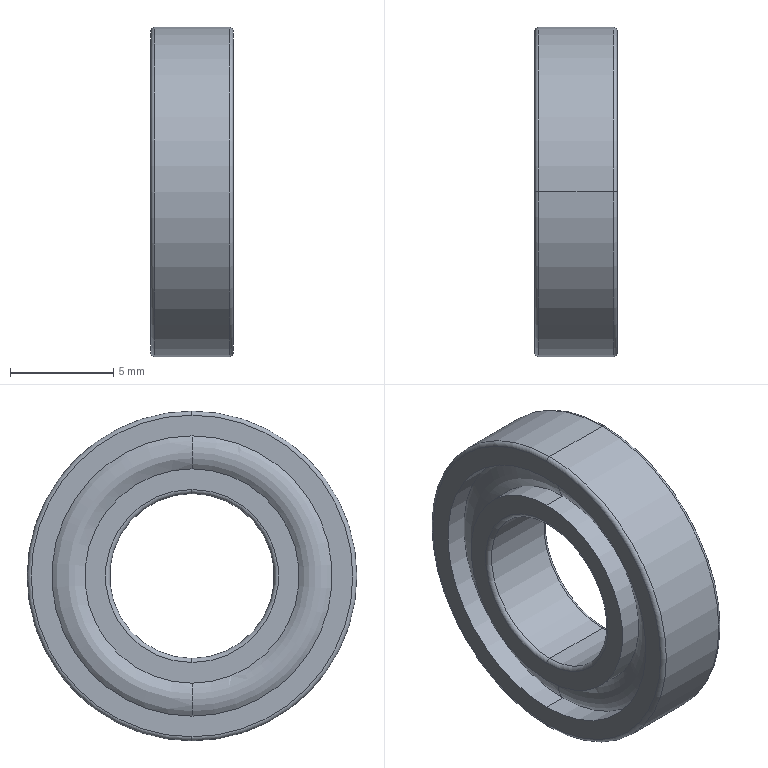Part | NX | features BREP 1 | 1 solid | 28 faces | box 4 x 16 x 16 mm | volume 493.797 mm3 | torus 12 | cylinder 12 | plane 4 | commonest cylinder face diameters 10.4 x4 13.6 x4 8 x2 16 x2
STEP:
#1=CARTESIAN_POINT('',(-2.,0.,-7.8));
#2=VERTEX_POINT('',#1);
#3=CARTESIAN_POINT('',(-2.,0.,7.8));
#4=VERTEX_POINT('',#3);
#5=CARTESIAN_POINT('',(-2.,0.,0.));
#6=DIRECTION('',(1.,0.,0.));
#7=DIRECTION('',(0.,0.,-1.));
#8=AXIS2_PLACEMENT_3D('',#5,#6,#7);
#9=CIRCLE('',#8,7.8);
#10=EDGE_CURVE('',#2,#4,#9,.T.);
#11=ORIENTED_EDGE('',*,*,#10,.T.);
#12=CARTESIAN_POINT('',(-1.8,0.,8.));
#13=VERTEX_POINT('',#12);
#14=CARTESIAN_POINT('',(-1.8,0.,7.8));
#15=DIRECTION('',(0.,1.,0.));
#16=DIRECTION('',(0.,0.,1.));
#17=AXIS2_PLACEMENT_3D('',#14,#15,#16);
#18=CIRCLE('',#17,0.2);
#19=EDGE_CURVE('',#4,#13,#18,.T.);
#20=ORIENTED_EDGE('',*,*,#19,.T.);
#21=CARTESIAN_POINT('',(-1.8,0.,-8.));
#22=VERTEX_POINT('',#21);
#23=CARTESIAN_POINT('',(-1.8,0.,0.));
#24=DIRECTION('',(1.,0.,0.));
#25=DIRECTION('',(0.,0.,-1.));
#26=AXIS2_PLACEMENT_3D('',#23,#24,#25);
#27=CIRCLE('',#26,8.);
#28=EDGE_CURVE('',#22,#13,#27,.T.);
#29=ORIENTED_EDGE('',*,*,#28,.F.);
#30=CARTESIAN_POINT('',(-1.8,0.,-7.8));
#31=DIRECTION('',(0.,-1.,0.));
#32=DIRECTION('',(0.,0.,-1.));
#33=AXIS2_PLACEMENT_3D('',#30,#31,#32);
#34=CIRCLE('',#33,0.2);
#35=EDGE_CURVE('',#2,#22,#34,.T.);
#36=ORIENTED_EDGE('',*,*,#35,.F.);
#37=EDGE_LOOP('',(#11,#20,#29,#36));
#38=FACE_BOUND('',#37,.T.);
#39=CARTESIAN_POINT('',(-1.8,0.,0.));
#40=DIRECTION('',(1.,0.,0.));
#41=DIRECTION('',(0.,0.,-1.));
#42=AXIS2_PLACEMENT_3D('',#39,#40,#41);
#43=TOROIDAL_SURFACE('',#42,7.8,0.2);
#44=ADVANCED_FACE('',(#38),#43,.T.);
#45=ORIENTED_EDGE('',*,*,#28,.T.);
#46=CARTESIAN_POINT('',(1.8,0.,8.));
#47=VERTEX_POINT('',#46);
#48=CARTESIAN_POINT('',(-20.638,0.,8.));
#49=DIRECTION('',(1.,0.,0.));
#50=VECTOR('',#49,1000.);
#51=LINE('',#48,#50);
#52=EDGE_CURVE('',#13,#47,#51,.T.);
#53=ORIENTED_EDGE('',*,*,#52,.T.);
#54=CARTESIAN_POINT('',(1.8,0.,-8.));
#55=VERTEX_POINT('',#54);
#56=CARTESIAN_POINT('',(1.8,0.,0.));
#57=DIRECTION('',(1.,0.,0.));
#58=DIRECTION('',(0.,0.,-1.));
#59=AXIS2_PLACEMENT_3D('',#56,#57,#58);
#60=CIRCLE('',#59,8.);
#61=EDGE_CURVE('',#55,#47,#60,.T.);
#62=ORIENTED_EDGE('',*,*,#61,.F.);
#63=CARTESIAN_POINT('',(-20.638,0.,-8.));
#64=DIRECTION('',(1.,0.,0.));
#65=VECTOR('',#64,1000.);
#66=LINE('',#63,#65);
#67=EDGE_CURVE('',#22,#55,#66,.T.);
#68=ORIENTED_EDGE('',*,*,#67,.F.);
#69=EDGE_LOOP('',(#45,#53,#62,#68));
#70=FACE_BOUND('',#69,.T.);
#71=CARTESIAN_POINT('',(-20.638,0.,0.));
#72=DIRECTION('',(1.,0.,0.));
#73=DIRECTION('',(0.,0.,-1.));
#74=AXIS2_PLACEMENT_3D('',#71,#72,#73);
#75=CYLINDRICAL_SURFACE('',#74,8.);
#76=ADVANCED_FACE('',(#70),#75,.T.);
#77=ORIENTED_EDGE('',*,*,#61,.T.);
#78=CARTESIAN_POINT('',(2.,0.,7.8));
#79=VERTEX_POINT('',#78);
#80=CARTESIAN_POINT('',(1.8,0.,7.8));
#81=DIRECTION('',(0.,1.,0.));
#82=DIRECTION('',(0.,0.,1.));
#83=AXIS2_PLACEMENT_3D('',#80,#81,#82);
#84=CIRCLE('',#83,0.2);
#85=EDGE_CURVE('',#47,#79,#84,.T.);
#86=ORIENTED_EDGE('',*,*,#85,.T.);
#87=CARTESIAN_POINT('',(2.,0.,-7.8));
#88=VERTEX_POINT('',#87);
#89=CARTESIAN_POINT('',(2.,0.,0.));
#90=DIRECTION('',(1.,0.,0.));
#91=DIRECTION('',(0.,0.,-1.));
#92=AXIS2_PLACEMENT_3D('',#89,#90,#91);
#93=CIRCLE('',#92,7.8);
#94=EDGE_CURVE('',#88,#79,#93,.T.);
#95=ORIENTED_EDGE('',*,*,#94,.F.);
#96=CARTESIAN_POINT('',(1.8,0.,-7.8));
#97=DIRECTION('',(0.,-1.,0.));
#98=DIRECTION('',(0.,0.,-1.));
#99=AXIS2_PLACEMENT_3D('',#96,#97,#98);
#100=CIRCLE('',#99,0.2);
#101=EDGE_CURVE('',#55,#88,#100,.T.);
#102=ORIENTED_EDGE('',*,*,#101,.F.);
#103=EDGE_LOOP('',(#77,#86,#95,#102));
#104=FACE_BOUND('',#103,.T.);
#105=CARTESIAN_POINT('',(1.8,0.,0.));
#106=DIRECTION('',(1.,0.,0.));
#107=DIRECTION('',(0.,0.,-1.));
#108=AXIS2_PLACEMENT_3D('',#105,#106,#107);
#109=TOROIDAL_SURFACE('',#108,7.8,0.2);
#110=ADVANCED_FACE('',(#104),#109,.T.);
#111=CARTESIAN_POINT('',(-2.,0.,6.8));
#112=VERTEX_POINT('',#111);
#113=CARTESIAN_POINT('',(-2.,0.,-6.8));
#114=VERTEX_POINT('',#113);
#115=CARTESIAN_POINT('',(-2.,0.,0.));
#116=DIRECTION('',(1.,0.,0.));
#117=DIRECTION('',(0.,0.,-1.));
#118=AXIS2_PLACEMENT_3D('',#115,#116,#117);
#119=CIRCLE('',#118,6.8);
#120=EDGE_CURVE('',#112,#114,#119,.T.);
#121=ORIENTED_EDGE('',*,*,#120,.F.);
#122=CARTESIAN_POINT('',(-0.8944,0.,6.8));
#123=VERTEX_POINT('',#122);
#124=CARTESIAN_POINT('',(-20.638,0.,6.8));
#125=DIRECTION('',(1.,0.,0.));
#126=VECTOR('',#125,1000.);
#127=LINE('',#124,#126);
#128=EDGE_CURVE('',#112,#123,#127,.T.);
#129=ORIENTED_EDGE('',*,*,#128,.T.);
#130=CARTESIAN_POINT('',(-0.8944,0.,-6.8));
#131=VERTEX_POINT('',#130);
#132=CARTESIAN_POINT('',(-0.8944,0.,0.));
#133=DIRECTION('',(-1.,0.,0.));
#134=DIRECTION('',(0.,0.,-1.));
#135=AXIS2_PLACEMENT_3D('',#132,#133,#134);
#136=CIRCLE('',#135,6.8);
#137=EDGE_CURVE('',#131,#123,#136,.T.);
#138=ORIENTED_EDGE('',*,*,#137,.F.);
#139=CARTESIAN_POINT('',(-20.638,0.,-6.8));
#140=DIRECTION('',(1.,0.,0.));
#141=VECTOR('',#140,1000.);
#142=LINE('',#139,#141);
#143=EDGE_CURVE('',#114,#131,#142,.T.);
#144=ORIENTED_EDGE('',*,*,#143,.F.);
#145=EDGE_LOOP('',(#121,#129,#138,#144));
#146=FACE_BOUND('',#145,.T.);
#147=CARTESIAN_POINT('',(-20.638,0.,0.));
#148=DIRECTION('',(1.,0.,0.));
#149=DIRECTION('',(0.,0.,-1.));
#150=AXIS2_PLACEMENT_3D('',#147,#148,#149);
#151=CYLINDRICAL_SURFACE('',#150,6.8);
#152=ADVANCED_FACE('',(#146),#151,.F.);
#153=CARTESIAN_POINT('',(0.8944,0.,6.8));
#154=VERTEX_POINT('',#153);
#155=CARTESIAN_POINT('',(0.8944,0.,-6.8));
#156=VERTEX_POINT('',#155);
#157=CARTESIAN_POINT('',(0.8944,0.,0.));
#158=DIRECTION('',(1.,0.,0.));
#159=DIRECTION('',(0.,0.,1.));
#160=AXIS2_PLACEMENT_3D('',#157,#158,#159);
#161=CIRCLE('',#160,6.8);
#162=EDGE_CURVE('',#154,#156,#161,.T.);
#163=ORIENTED_EDGE('',*,*,#162,.F.);
#164=CARTESIAN_POINT('',(2.,0.,6.8));
#165=VERTEX_POINT('',#164);
#166=CARTESIAN_POINT('',(-20.638,0.,6.8));
#167=DIRECTION('',(1.,0.,0.));
#168=VECTOR('',#167,1000.);
#169=LINE('',#166,#168);
#170=EDGE_CURVE('',#154,#165,#169,.T.);
#171=ORIENTED_EDGE('',*,*,#170,.T.);
#172=CARTESIAN_POINT('',(2.,0.,-6.8));
#173=VERTEX_POINT('',#172);
#174=CARTESIAN_POINT('',(2.,0.,0.));
#175=DIRECTION('',(1.,0.,0.));
#176=DIRECTION('',(0.,0.,-1.));
#177=AXIS2_PLACEMENT_3D('',#174,#175,#176);
#178=CIRCLE('',#177,6.8);
#179=EDGE_CURVE('',#165,#173,#178,.T.);
#180=ORIENTED_EDGE('',*,*,#179,.T.);
#181=CARTESIAN_POINT('',(-20.638,0.,-6.8));
#182=DIRECTION('',(1.,0.,0.));
#183=VECTOR('',#182,1000.);
#184=LINE('',#181,#183);
#185=EDGE_CURVE('',#156,#173,#184,.T.);
#186=ORIENTED_EDGE('',*,*,#185,.F.);
#187=EDGE_LOOP('',(#163,#171,#180,#186));
#188=FACE_BOUND('',#187,.T.);
#189=CARTESIAN_POINT('',(-20.638,0.,0.));
#190=DIRECTION('',(1.,0.,0.));
#191=DIRECTION('',(0.,0.,-1.));
#192=AXIS2_PLACEMENT_3D('',#189,#190,#191);
#193=CYLINDRICAL_SURFACE('',#192,6.8);
#194=ADVANCED_FACE('',(#188),#193,.F.);
#195=CARTESIAN_POINT('',(-0.8944,0.,0.));
#196=DIRECTION('',(-1.,0.,0.));
#197=DIRECTION('',(0.,0.,-1.));
#198=AXIS2_PLACEMENT_3D('',#195,#196,#197);
#199=CIRCLE('',#198,6.8);
#200=EDGE_CURVE('',#123,#131,#199,.T.);
#201=ORIENTED_EDGE('',*,*,#200,.T.);
#202=CARTESIAN_POINT('',(-0.8944,0.,-5.2));
#203=VERTEX_POINT('',#202);
#204=CARTESIAN_POINT('',(0.,0.,-6.));
#205=DIRECTION('',(0.,1.,0.));
#206=DIRECTION('',(0.,0.,1.));
#207=AXIS2_PLACEMENT_3D('',#204,#205,#206);
#208=CIRCLE('',#207,1.2);
#209=EDGE_CURVE('',#203,#131,#208,.F.);
#210=ORIENTED_EDGE('',*,*,#209,.F.);
#211=CARTESIAN_POINT('',(-0.8944,0.,5.2));
#212=VERTEX_POINT('',#211);
#213=CARTESIAN_POINT('',(-0.8944,0.,0.));
#214=DIRECTION('',(1.,0.,0.));
#215=DIRECTION('',(0.,0.,-1.));
#216=AXIS2_PLACEMENT_3D('',#213,#214,#215);
#217=CIRCLE('',#216,5.2);
#218=EDGE_CURVE('',#203,#212,#217,.T.);
#219=ORIENTED_EDGE('',*,*,#218,.T.);
#220=CARTESIAN_POINT('',(0.,0.,6.));
#221=DIRECTION('',(0.,-1.,0.));
#222=DIRECTION('',(0.,0.,-1.));
#223=AXIS2_PLACEMENT_3D('',#220,#221,#222);
#224=CIRCLE('',#223,1.2);
#225=EDGE_CURVE('',#212,#123,#224,.F.);
#226=ORIENTED_EDGE('',*,*,#225,.T.);
#227=EDGE_LOOP('',(#201,#210,#219,#226));
#228=FACE_BOUND('',#227,.T.);
#229=CARTESIAN_POINT('',(0.,0.,0.));
#230=DIRECTION('',(-1.,0.,0.));
#231=DIRECTION('',(0.,0.,1.));
#232=AXIS2_PLACEMENT_3D('',#229,#230,#231);
#233=TOROIDAL_SURFACE('',#232,6.,1.2);
#234=ADVANCED_FACE('',(#228),#233,.T.);
#235=CARTESIAN_POINT('',(-1.8,0.,-4.));
#236=VERTEX_POINT('',#235);
#237=CARTESIAN_POINT('',(-1.8,0.,4.));
#238=VERTEX_POINT('',#237);
#239=CARTESIAN_POINT('',(-1.8,0.,0.));
#240=DIRECTION('',(1.,0.,0.));
#241=DIRECTION('',(0.,0.,-1.));
#242=AXIS2_PLACEMENT_3D('',#239,#240,#241);
#243=CIRCLE('',#242,4.);
#244=EDGE_CURVE('',#236,#238,#243,.T.);
#245=ORIENTED_EDGE('',*,*,#244,.T.);
#246=CARTESIAN_POINT('',(-2.,0.,4.2));
#247=VERTEX_POINT('',#246);
#248=CARTESIAN_POINT('',(-1.8,0.,4.2));
#249=DIRECTION('',(0.,1.,0.));
#250=DIRECTION('',(0.,0.,1.));
#251=AXIS2_PLACEMENT_3D('',#248,#249,#250);
#252=CIRCLE('',#251,0.2);
#253=EDGE_CURVE('',#238,#247,#252,.T.);
#254=ORIENTED_EDGE('',*,*,#253,.T.);
#255=CARTESIAN_POINT('',(-2.,0.,-4.2));
#256=VERTEX_POINT('',#255);
#257=CARTESIAN_POINT('',(-2.,0.,0.));
#258=DIRECTION('',(1.,0.,0.));
#259=DIRECTION('',(0.,0.,-1.));
#260=AXIS2_PLACEMENT_3D('',#257,#258,#259);
#261=CIRCLE('',#260,4.2);
#262=EDGE_CURVE('',#256,#247,#261,.T.);
#263=ORIENTED_EDGE('',*,*,#262,.F.);
#264=CARTESIAN_POINT('',(-1.8,0.,-4.2));
#265=DIRECTION('',(0.,-1.,0.));
#266=DIRECTION('',(0.,0.,-1.));
#267=AXIS2_PLACEMENT_3D('',#264,#265,#266);
#268=CIRCLE('',#267,0.2);
#269=EDGE_CURVE('',#236,#256,#268,.T.);
#270=ORIENTED_EDGE('',*,*,#269,.F.);
#271=EDGE_LOOP('',(#245,#254,#263,#270));
#272=FACE_BOUND('',#271,.T.);
#273=CARTESIAN_POINT('',(-1.8,0.,0.));
#274=DIRECTION('',(1.,0.,0.));
#275=DIRECTION('',(0.,0.,-1.));
#276=AXIS2_PLACEMENT_3D('',#273,#274,#275);
#277=TOROIDAL_SURFACE('',#276,4.2,0.2);
#278=ADVANCED_FACE('',(#272),#277,.T.);
#279=CARTESIAN_POINT('',(-1.8,0.,0.));
#280=DIRECTION('',(1.,0.,0.));
#281=DIRECTION('',(0.,0.,-1.));
#282=AXIS2_PLACEMENT_3D('',#279,#280,#281);
#283=CIRCLE('',#282,4.);
#284=EDGE_CURVE('',#238,#236,#283,.T.);
#285=ORIENTED_EDGE('',*,*,#284,.F.);
#286=CARTESIAN_POINT('',(1.8,0.,4.));
#287=VERTEX_POINT('',#286);
#288=CARTESIAN_POINT('',(-20.638,0.,4.));
#289=DIRECTION('',(1.,0.,0.));
#290=VECTOR('',#289,1000.);
#291=LINE('',#288,#290);
#292=EDGE_CURVE('',#238,#287,#291,.T.);
#293=ORIENTED_EDGE('',*,*,#292,.T.);
#294=CARTESIAN_POINT('',(1.8,0.,-4.));
#295=VERTEX_POINT('',#294);
#296=CARTESIAN_POINT('',(1.8,0.,0.));
#297=DIRECTION('',(1.,0.,0.));
#298=DIRECTION('',(0.,0.,-1.));
#299=AXIS2_PLACEMENT_3D('',#296,#297,#298);
#300=CIRCLE('',#299,4.);
#301=EDGE_CURVE('',#287,#295,#300,.T.);
#302=ORIENTED_EDGE('',*,*,#301,.T.);
#303=CARTESIAN_POINT('',(-20.638,0.,-4.));
#304=DIRECTION('',(1.,0.,0.));
#305=VECTOR('',#304,1000.);
#306=LINE('',#303,#305);
#307=EDGE_CURVE('',#236,#295,#306,.T.);
#308=ORIENTED_EDGE('',*,*,#307,.F.);
#309=EDGE_LOOP('',(#285,#293,#302,#308));
#310=FACE_BOUND('',#309,.T.);
#311=CARTESIAN_POINT('',(-20.638,0.,0.));
#312=DIRECTION('',(1.,0.,0.));
#313=DIRECTION('',(0.,0.,-1.));
#314=AXIS2_PLACEMENT_3D('',#311,#312,#313);
#315=CYLINDRICAL_SURFACE('',#314,4.);
#316=ADVANCED_FACE('',(#310),#315,.F.);
#317=CARTESIAN_POINT('',(2.,0.,-4.2));
#318=VERTEX_POINT('',#317);
#319=CARTESIAN_POINT('',(2.,0.,4.2));
#320=VERTEX_POINT('',#319);
#321=CARTESIAN_POINT('',(2.,0.,0.));
#322=DIRECTION('',(1.,0.,0.));
#323=DIRECTION('',(0.,0.,-1.));
#324=AXIS2_PLACEMENT_3D('',#321,#322,#323);
#325=CIRCLE('',#324,4.2);
#326=EDGE_CURVE('',#318,#320,#325,.T.);
#327=ORIENTED_EDGE('',*,*,#326,.T.);
#328=CARTESIAN_POINT('',(1.8,0.,4.2));
#329=DIRECTION('',(0.,1.,0.));
#330=DIRECTION('',(0.,0.,1.));
#331=AXIS2_PLACEMENT_3D('',#328,#329,#330);
#332=CIRCLE('',#331,0.2);
#333=EDGE_CURVE('',#320,#287,#332,.T.);
#334=ORIENTED_EDGE('',*,*,#333,.T.);
#335=CARTESIAN_POINT('',(1.8,0.,0.));
#336=DIRECTION('',(1.,0.,0.));
#337=DIRECTION('',(0.,0.,-1.));
#338=AXIS2_PLACEMENT_3D('',#335,#336,#337);
#339=CIRCLE('',#338,4.);
#340=EDGE_CURVE('',#295,#287,#339,.T.);
#341=ORIENTED_EDGE('',*,*,#340,.F.);
#342=CARTESIAN_POINT('',(1.8,0.,-4.2));
#343=DIRECTION('',(0.,-1.,0.));
#344=DIRECTION('',(0.,0.,-1.));
#345=AXIS2_PLACEMENT_3D('',#342,#343,#344);
#346=CIRCLE('',#345,0.2);
#347=EDGE_CURVE('',#318,#295,#346,.T.);
#348=ORIENTED_EDGE('',*,*,#347,.F.);
#349=EDGE_LOOP('',(#327,#334,#341,#348));
#350=FACE_BOUND('',#349,.T.);
#351=CARTESIAN_POINT('',(1.8,0.,0.));
#352=DIRECTION('',(1.,0.,0.));
#353=DIRECTION('',(0.,0.,-1.));
#354=AXIS2_PLACEMENT_3D('',#351,#352,#353);
#355=TOROIDAL_SURFACE('',#354,4.2,0.2);
#356=ADVANCED_FACE('',(#350),#355,.T.);
#357=CARTESIAN_POINT('',(-2.,0.,-5.2));
#358=VERTEX_POINT('',#357);
#359=CARTESIAN_POINT('',(-2.,0.,5.2));
#360=VERTEX_POINT('',#359);
#361=CARTESIAN_POINT('',(-2.,0.,0.));
#362=DIRECTION('',(1.,0.,0.));
#363=DIRECTION('',(0.,0.,-1.));
#364=AXIS2_PLACEMENT_3D('',#361,#362,#363);
#365=CIRCLE('',#364,5.2);
#366=EDGE_CURVE('',#358,#360,#365,.T.);
#367=ORIENTED_EDGE('',*,*,#366,.T.);
#368=CARTESIAN_POINT('',(-20.638,0.,5.2));
#369=DIRECTION('',(1.,0.,0.));
#370=VECTOR('',#369,1000.);
#371=LINE('',#368,#370);
#372=EDGE_CURVE('',#360,#212,#371,.T.);
#373=ORIENTED_EDGE('',*,*,#372,.T.);
#374=ORIENTED_EDGE('',*,*,#218,.F.);
#375=CARTESIAN_POINT('',(-20.638,0.,-5.2));
#376=DIRECTION('',(1.,0.,0.));
#377=VECTOR('',#376,1000.);
#378=LINE('',#375,#377);
#379=EDGE_CURVE('',#358,#203,#378,.T.);
#380=ORIENTED_EDGE('',*,*,#379,.F.);
#381=EDGE_LOOP('',(#367,#373,#374,#380));
#382=FACE_BOUND('',#381,.T.);
#383=CARTESIAN_POINT('',(-20.638,0.,0.));
#384=DIRECTION('',(1.,0.,0.));
#385=DIRECTION('',(0.,0.,-1.));
#386=AXIS2_PLACEMENT_3D('',#383,#384,#385);
#387=CYLINDRICAL_SURFACE('',#386,5.2);
#388=ADVANCED_FACE('',(#382),#387,.T.);
#389=CARTESIAN_POINT('',(0.8944,0.,5.2));
#390=VERTEX_POINT('',#389);
#391=CARTESIAN_POINT('',(0.8944,0.,-5.2));
#392=VERTEX_POINT('',#391);
#393=CARTESIAN_POINT('',(0.8944,0.,0.));
#394=DIRECTION('',(-1.,0.,0.));
#395=DIRECTION('',(0.,0.,1.));
#396=AXIS2_PLACEMENT_3D('',#393,#394,#395);
#397=CIRCLE('',#396,5.2);
#398=EDGE_CURVE('',#390,#392,#397,.T.);
#399=ORIENTED_EDGE('',*,*,#398,.F.);
#400=CARTESIAN_POINT('',(2.,0.,5.2));
#401=VERTEX_POINT('',#400);
#402=CARTESIAN_POINT('',(-20.638,0.,5.2));
#403=DIRECTION('',(1.,0.,0.));
#404=VECTOR('',#403,1000.);
#405=LINE('',#402,#404);
#406=EDGE_CURVE('',#390,#401,#405,.T.);
#407=ORIENTED_EDGE('',*,*,#406,.T.);
#408=CARTESIAN_POINT('',(2.,0.,-5.2));
#409=VERTEX_POINT('',#408);
#410=CARTESIAN_POINT('',(2.,0.,0.));
#411=DIRECTION('',(1.,0.,0.));
#412=DIRECTION('',(0.,0.,-1.));
#413=AXIS2_PLACEMENT_3D('',#410,#411,#412);
#414=CIRCLE('',#413,5.2);
#415=EDGE_CURVE('',#409,#401,#414,.T.);
#416=ORIENTED_EDGE('',*,*,#415,.F.);
#417=CARTESIAN_POINT('',(-20.638,0.,-5.2));
#418=DIRECTION('',(1.,0.,0.));
#419=VECTOR('',#418,1000.);
#420=LINE('',#417,#419);
#421=EDGE_CURVE('',#392,#409,#420,.T.);
#422=ORIENTED_EDGE('',*,*,#421,.F.);
#423=EDGE_LOOP('',(#399,#407,#416,#422));
#424=FACE_BOUND('',#423,.T.);
#425=CARTESIAN_POINT('',(-20.638,0.,0.));
#426=DIRECTION('',(1.,0.,0.));
#427=DIRECTION('',(0.,0.,-1.));
#428=AXIS2_PLACEMENT_3D('',#425,#426,#427);
#429=CYLINDRICAL_SURFACE('',#428,5.2);
#430=ADVANCED_FACE('',(#424),#429,.T.);
#431=ORIENTED_EDGE('',*,*,#398,.T.);
#432=CARTESIAN_POINT('',(0.,0.,-6.));
#433=DIRECTION('',(0.,1.,0.));
#434=DIRECTION('',(0.,0.,1.));
#435=AXIS2_PLACEMENT_3D('',#432,#433,#434);
#436=CIRCLE('',#435,1.2);
#437=EDGE_CURVE('',#156,#392,#436,.F.);
#438=ORIENTED_EDGE('',*,*,#437,.F.);
#439=CARTESIAN_POINT('',(0.8944,0.,0.));
#440=DIRECTION('',(1.,0.,0.));
#441=DIRECTION('',(0.,0.,1.));
#442=AXIS2_PLACEMENT_3D('',#439,#440,#441);
#443=CIRCLE('',#442,6.8);
#444=EDGE_CURVE('',#156,#154,#443,.T.);
#445=ORIENTED_EDGE('',*,*,#444,.T.);
#446=CARTESIAN_POINT('',(0.,0.,6.));
#447=DIRECTION('',(0.,-1.,0.));
#448=DIRECTION('',(0.,0.,-1.));
#449=AXIS2_PLACEMENT_3D('',#446,#447,#448);
#450=CIRCLE('',#449,1.2);
#451=EDGE_CURVE('',#154,#390,#450,.F.);
#452=ORIENTED_EDGE('',*,*,#451,.T.);
#453=EDGE_LOOP('',(#431,#438,#445,#452));
#454=FACE_BOUND('',#453,.T.);
#455=CARTESIAN_POINT('',(0.,0.,0.));
#456=DIRECTION('',(-1.,0.,0.));
#457=DIRECTION('',(0.,0.,1.));
#458=AXIS2_PLACEMENT_3D('',#455,#456,#457);
#459=TOROIDAL_SURFACE('',#458,6.,1.2);
#460=ADVANCED_FACE('',(#454),#459,.T.);
#461=ORIENTED_EDGE('',*,*,#437,.T.);
#462=CARTESIAN_POINT('',(0.8944,0.,0.));
#463=DIRECTION('',(-1.,0.,0.));
#464=DIRECTION('',(0.,0.,1.));
#465=AXIS2_PLACEMENT_3D('',#462,#463,#464);
#466=CIRCLE('',#465,5.2);
#467=EDGE_CURVE('',#392,#390,#466,.T.);
#468=ORIENTED_EDGE('',*,*,#467,.T.);
#469=ORIENTED_EDGE('',*,*,#451,.F.);
#470=ORIENTED_EDGE('',*,*,#162,.T.);
#471=EDGE_LOOP('',(#461,#468,#469,#470));
#472=FACE_BOUND('',#471,.T.);
#473=CARTESIAN_POINT('',(0.,0.,0.));
#474=DIRECTION('',(-1.,0.,0.));
#475=DIRECTION('',(0.,0.,1.));
#476=AXIS2_PLACEMENT_3D('',#473,#474,#475);
#477=TOROIDAL_SURFACE('',#476,6.,1.2);
#478=ADVANCED_FACE('',(#472),#477,.T.);
#479=ORIENTED_EDGE('',*,*,#406,.F.);
#480=ORIENTED_EDGE('',*,*,#467,.F.);
#481=ORIENTED_EDGE('',*,*,#421,.T.);
#482=CARTESIAN_POINT('',(2.,0.,0.));
#483=DIRECTION('',(1.,0.,0.));
#484=DIRECTION('',(0.,0.,-1.));
#485=AXIS2_PLACEMENT_3D('',#482,#483,#484);
#486=CIRCLE('',#485,5.2);
#487=EDGE_CURVE('',#401,#409,#486,.T.);
#488=ORIENTED_EDGE('',*,*,#487,.F.);
#489=EDGE_LOOP('',(#479,#480,#481,#488));
#490=FACE_BOUND('',#489,.T.);
#491=CARTESIAN_POINT('',(-20.638,0.,0.));
#492=DIRECTION('',(1.,0.,0.));
#493=DIRECTION('',(0.,0.,-1.));
#494=AXIS2_PLACEMENT_3D('',#491,#492,#493);
#495=CYLINDRICAL_SURFACE('',#494,5.2);
#496=ADVANCED_FACE('',(#490),#495,.T.);
#497=ORIENTED_EDGE('',*,*,#372,.F.);
#498=CARTESIAN_POINT('',(-2.,0.,0.));
#499=DIRECTION('',(1.,0.,0.));
#500=DIRECTION('',(0.,0.,-1.));
#501=AXIS2_PLACEMENT_3D('',#498,#499,#500);
#502=CIRCLE('',#501,5.2);
#503=EDGE_CURVE('',#360,#358,#502,.T.);
#504=ORIENTED_EDGE('',*,*,#503,.T.);
#505=ORIENTED_EDGE('',*,*,#379,.T.);
#506=CARTESIAN_POINT('',(-0.8944,0.,0.));
#507=DIRECTION('',(1.,0.,0.));
#508=DIRECTION('',(0.,0.,-1.));
#509=AXIS2_PLACEMENT_3D('',#506,#507,#508);
#510=CIRCLE('',#509,5.2);
#511=EDGE_CURVE('',#212,#203,#510,.T.);
#512=ORIENTED_EDGE('',*,*,#511,.F.);
#513=EDGE_LOOP('',(#497,#504,#505,#512));
#514=FACE_BOUND('',#513,.T.);
#515=CARTESIAN_POINT('',(-20.638,0.,0.));
#516=DIRECTION('',(1.,0.,0.));
#517=DIRECTION('',(0.,0.,-1.));
#518=AXIS2_PLACEMENT_3D('',#515,#516,#517);
#519=CYLINDRICAL_SURFACE('',#518,5.2);
#520=ADVANCED_FACE('',(#514),#519,.T.);
#521=ORIENTED_EDGE('',*,*,#415,.T.);
#522=ORIENTED_EDGE('',*,*,#487,.T.);
#523=EDGE_LOOP('',(#521,#522));
#524=FACE_BOUND('',#523,.T.);
#525=ORIENTED_EDGE('',*,*,#326,.F.);
#526=CARTESIAN_POINT('',(2.,0.,0.));
#527=DIRECTION('',(1.,0.,0.));
#528=DIRECTION('',(0.,0.,-1.));
#529=AXIS2_PLACEMENT_3D('',#526,#527,#528);
#530=CIRCLE('',#529,4.2);
#531=EDGE_CURVE('',#320,#318,#530,.T.);
#532=ORIENTED_EDGE('',*,*,#531,.F.);
#533=EDGE_LOOP('',(#525,#532));
#534=FACE_BOUND('',#533,.T.);
#535=CARTESIAN_POINT('',(2.,4.2,0.));
#536=DIRECTION('',(1.,0.,0.));
#537=DIRECTION('',(0.,1.,0.));
#538=AXIS2_PLACEMENT_3D('',#535,#536,#537);
#539=PLANE('',#538);
#540=ADVANCED_FACE('',(#524,#534),#539,.T.);
#541=ORIENTED_EDGE('',*,*,#333,.F.);
#542=ORIENTED_EDGE('',*,*,#531,.T.);
#543=ORIENTED_EDGE('',*,*,#347,.T.);
#544=ORIENTED_EDGE('',*,*,#301,.F.);
#545=EDGE_LOOP('',(#541,#542,#543,#544));
#546=FACE_BOUND('',#545,.T.);
#547=CARTESIAN_POINT('',(1.8,0.,0.));
#548=DIRECTION('',(1.,0.,0.));
#549=DIRECTION('',(0.,0.,-1.));
#550=AXIS2_PLACEMENT_3D('',#547,#548,#549);
#551=TOROIDAL_SURFACE('',#550,4.2,0.2);
#552=ADVANCED_FACE('',(#546),#551,.T.);
#553=ORIENTED_EDGE('',*,*,#292,.F.);
#554=ORIENTED_EDGE('',*,*,#244,.F.);
#555=ORIENTED_EDGE('',*,*,#307,.T.);
#556=ORIENTED_EDGE('',*,*,#340,.T.);
#557=EDGE_LOOP('',(#553,#554,#555,#556));
#558=FACE_BOUND('',#557,.T.);
#559=CARTESIAN_POINT('',(-20.638,0.,0.));
#560=DIRECTION('',(1.,0.,0.));
#561=DIRECTION('',(0.,0.,-1.));
#562=AXIS2_PLACEMENT_3D('',#559,#560,#561);
#563=CYLINDRICAL_SURFACE('',#562,4.);
#564=ADVANCED_FACE('',(#558),#563,.F.);
#565=ORIENTED_EDGE('',*,*,#253,.F.);
#566=ORIENTED_EDGE('',*,*,#284,.T.);
#567=ORIENTED_EDGE('',*,*,#269,.T.);
#568=CARTESIAN_POINT('',(-2.,0.,0.));
#569=DIRECTION('',(1.,0.,0.));
#570=DIRECTION('',(0.,0.,-1.));
#571=AXIS2_PLACEMENT_3D('',#568,#569,#570);
#572=CIRCLE('',#571,4.2);
#573=EDGE_CURVE('',#247,#256,#572,.T.);
#574=ORIENTED_EDGE('',*,*,#573,.F.);
#575=EDGE_LOOP('',(#565,#566,#567,#574));
#576=FACE_BOUND('',#575,.T.);
#577=CARTESIAN_POINT('',(-1.8,0.,0.));
#578=DIRECTION('',(1.,0.,0.));
#579=DIRECTION('',(0.,0.,-1.));
#580=AXIS2_PLACEMENT_3D('',#577,#578,#579);
#581=TOROIDAL_SURFACE('',#580,4.2,0.2);
#582=ADVANCED_FACE('',(#576),#581,.T.);
#583=ORIENTED_EDGE('',*,*,#366,.F.);
#584=ORIENTED_EDGE('',*,*,#503,.F.);
#585=EDGE_LOOP('',(#583,#584));
#586=FACE_BOUND('',#585,.T.);
#587=ORIENTED_EDGE('',*,*,#262,.T.);
#588=ORIENTED_EDGE('',*,*,#573,.T.);
#589=EDGE_LOOP('',(#587,#588));
#590=FACE_BOUND('',#589,.T.);
#591=CARTESIAN_POINT('',(-2.,5.2,0.));
#592=DIRECTION('',(-1.,0.,0.));
#593=DIRECTION('',(0.,1.,0.));
#594=AXIS2_PLACEMENT_3D('',#591,#592,#593);
#595=PLANE('',#594);
#596=ADVANCED_FACE('',(#586,#590),#595,.T.);
#597=ORIENTED_EDGE('',*,*,#209,.T.);
#598=ORIENTED_EDGE('',*,*,#137,.T.);
#599=ORIENTED_EDGE('',*,*,#225,.F.);
#600=ORIENTED_EDGE('',*,*,#511,.T.);
#601=EDGE_LOOP('',(#597,#598,#599,#600));
#602=FACE_BOUND('',#601,.T.);
#603=CARTESIAN_POINT('',(0.,0.,0.));
#604=DIRECTION('',(-1.,0.,0.));
#605=DIRECTION('',(0.,0.,1.));
#606=AXIS2_PLACEMENT_3D('',#603,#604,#605);
#607=TOROIDAL_SURFACE('',#606,6.,1.2);
#608=ADVANCED_FACE('',(#602),#607,.T.);
#609=ORIENTED_EDGE('',*,*,#170,.F.);
#610=ORIENTED_EDGE('',*,*,#444,.F.);
#611=ORIENTED_EDGE('',*,*,#185,.T.);
#612=CARTESIAN_POINT('',(2.,0.,0.));
#613=DIRECTION('',(1.,0.,0.));
#614=DIRECTION('',(0.,0.,-1.));
#615=AXIS2_PLACEMENT_3D('',#612,#613,#614);
#616=CIRCLE('',#615,6.8);
#617=EDGE_CURVE('',#173,#165,#616,.T.);
#618=ORIENTED_EDGE('',*,*,#617,.T.);
#619=EDGE_LOOP('',(#609,#610,#611,#618));
#620=FACE_BOUND('',#619,.T.);
#621=CARTESIAN_POINT('',(-20.638,0.,0.));
#622=DIRECTION('',(1.,0.,0.));
#623=DIRECTION('',(0.,0.,-1.));
#624=AXIS2_PLACEMENT_3D('',#621,#622,#623);
#625=CYLINDRICAL_SURFACE('',#624,6.8);
#626=ADVANCED_FACE('',(#620),#625,.F.);
#627=ORIENTED_EDGE('',*,*,#128,.F.);
#628=CARTESIAN_POINT('',(-2.,0.,0.));
#629=DIRECTION('',(1.,0.,0.));
#630=DIRECTION('',(0.,0.,-1.));
#631=AXIS2_PLACEMENT_3D('',#628,#629,#630);
#632=CIRCLE('',#631,6.8);
#633=EDGE_CURVE('',#114,#112,#632,.T.);
#634=ORIENTED_EDGE('',*,*,#633,.F.);
#635=ORIENTED_EDGE('',*,*,#143,.T.);
#636=ORIENTED_EDGE('',*,*,#200,.F.);
#637=EDGE_LOOP('',(#627,#634,#635,#636));
#638=FACE_BOUND('',#637,.T.);
#639=CARTESIAN_POINT('',(-20.638,0.,0.));
#640=DIRECTION('',(1.,0.,0.));
#641=DIRECTION('',(0.,0.,-1.));
#642=AXIS2_PLACEMENT_3D('',#639,#640,#641);
#643=CYLINDRICAL_SURFACE('',#642,6.8);
#644=ADVANCED_FACE('',(#638),#643,.F.);
#645=ORIENTED_EDGE('',*,*,#94,.T.);
#646=CARTESIAN_POINT('',(2.,0.,0.));
#647=DIRECTION('',(1.,0.,0.));
#648=DIRECTION('',(0.,0.,-1.));
#649=AXIS2_PLACEMENT_3D('',#646,#647,#648);
#650=CIRCLE('',#649,7.8);
#651=EDGE_CURVE('',#79,#88,#650,.T.);
#652=ORIENTED_EDGE('',*,*,#651,.T.);
#653=EDGE_LOOP('',(#645,#652));
#654=FACE_BOUND('',#653,.T.);
#655=ORIENTED_EDGE('',*,*,#617,.F.);
#656=ORIENTED_EDGE('',*,*,#179,.F.);
#657=EDGE_LOOP('',(#655,#656));
#658=FACE_BOUND('',#657,.T.);
#659=CARTESIAN_POINT('',(2.,7.8,0.));
#660=DIRECTION('',(1.,0.,0.));
#661=DIRECTION('',(0.,1.,0.));
#662=AXIS2_PLACEMENT_3D('',#659,#660,#661);
#663=PLANE('',#662);
#664=ADVANCED_FACE('',(#654,#658),#663,.T.);
#665=ORIENTED_EDGE('',*,*,#85,.F.);
#666=CARTESIAN_POINT('',(1.8,0.,0.));
#667=DIRECTION('',(1.,0.,0.));
#668=DIRECTION('',(0.,0.,-1.));
#669=AXIS2_PLACEMENT_3D('',#666,#667,#668);
#670=CIRCLE('',#669,8.);
#671=EDGE_CURVE('',#47,#55,#670,.T.);
#672=ORIENTED_EDGE('',*,*,#671,.T.);
#673=ORIENTED_EDGE('',*,*,#101,.T.);
#674=ORIENTED_EDGE('',*,*,#651,.F.);
#675=EDGE_LOOP('',(#665,#672,#673,#674));
#676=FACE_BOUND('',#675,.T.);
#677=CARTESIAN_POINT('',(1.8,0.,0.));
#678=DIRECTION('',(1.,0.,0.));
#679=DIRECTION('',(0.,0.,-1.));
#680=AXIS2_PLACEMENT_3D('',#677,#678,#679);
#681=TOROIDAL_SURFACE('',#680,7.8,0.2);
#682=ADVANCED_FACE('',(#676),#681,.T.);
#683=ORIENTED_EDGE('',*,*,#52,.F.);
#684=CARTESIAN_POINT('',(-1.8,0.,0.));
#685=DIRECTION('',(1.,0.,0.));
#686=DIRECTION('',(0.,0.,-1.));
#687=AXIS2_PLACEMENT_3D('',#684,#685,#686);
#688=CIRCLE('',#687,8.);
#689=EDGE_CURVE('',#13,#22,#688,.T.);
#690=ORIENTED_EDGE('',*,*,#689,.T.);
#691=ORIENTED_EDGE('',*,*,#67,.T.);
#692=ORIENTED_EDGE('',*,*,#671,.F.);
#693=EDGE_LOOP('',(#683,#690,#691,#692));
#694=FACE_BOUND('',#693,.T.);
#695=CARTESIAN_POINT('',(-20.638,0.,0.));
#696=DIRECTION('',(1.,0.,0.));
#697=DIRECTION('',(0.,0.,-1.));
#698=AXIS2_PLACEMENT_3D('',#695,#696,#697);
#699=CYLINDRICAL_SURFACE('',#698,8.);
#700=ADVANCED_FACE('',(#694),#699,.T.);
#701=ORIENTED_EDGE('',*,*,#19,.F.);
#702=CARTESIAN_POINT('',(-2.,0.,0.));
#703=DIRECTION('',(1.,0.,0.));
#704=DIRECTION('',(0.,0.,-1.));
#705=AXIS2_PLACEMENT_3D('',#702,#703,#704);
#706=CIRCLE('',#705,7.8);
#707=EDGE_CURVE('',#4,#2,#706,.T.);
#708=ORIENTED_EDGE('',*,*,#707,.T.);
#709=ORIENTED_EDGE('',*,*,#35,.T.);
#710=ORIENTED_EDGE('',*,*,#689,.F.);
#711=EDGE_LOOP('',(#701,#708,#709,#710));
#712=FACE_BOUND('',#711,.T.);
#713=CARTESIAN_POINT('',(-1.8,0.,0.));
#714=DIRECTION('',(1.,0.,0.));
#715=DIRECTION('',(0.,0.,-1.));
#716=AXIS2_PLACEMENT_3D('',#713,#714,#715);
#717=TOROIDAL_SURFACE('',#716,7.8,0.2);
#718=ADVANCED_FACE('',(#712),#717,.T.);
#719=ORIENTED_EDGE('',*,*,#10,.F.);
#720=ORIENTED_EDGE('',*,*,#707,.F.);
#721=EDGE_LOOP('',(#719,#720));
#722=FACE_BOUND('',#721,.T.);
#723=ORIENTED_EDGE('',*,*,#633,.T.);
#724=ORIENTED_EDGE('',*,*,#120,.T.);
#725=EDGE_LOOP('',(#723,#724));
#726=FACE_BOUND('',#725,.T.);
#727=CARTESIAN_POINT('',(-2.,6.8,0.));
#728=DIRECTION('',(-1.,0.,0.));
#729=DIRECTION('',(0.,1.,0.));
#730=AXIS2_PLACEMENT_3D('',#727,#728,#729);
#731=PLANE('',#730);
#732=ADVANCED_FACE('',(#722,#726),#731,.T.);
#733=CLOSED_SHELL('',(#44,#76,#110,#152,#194,#234,#278,#316,#356,#388,#430,#460,#478,#496,#520,#540,#552,#564,#582,#596,#608,#626,#644,#664,#682,#700,#718,#732));
#734=MANIFOLD_SOLID_BREP('',#733);
#735=(LENGTH_UNIT()NAMED_UNIT(*)SI_UNIT(.MILLI.,.METRE.));
#736=UNCERTAINTY_MEASURE_WITH_UNIT(LENGTH_MEASURE(0.00001),#735,'','');
#737=(NAMED_UNIT(*)PLANE_ANGLE_UNIT()SI_UNIT($,.RADIAN.));
#738=(NAMED_UNIT(*)SI_UNIT($,.STERADIAN.)SOLID_ANGLE_UNIT());
#739=(GEOMETRIC_REPRESENTATION_CONTEXT(3)GLOBAL_UNCERTAINTY_ASSIGNED_CONTEXT((#736))GLOBAL_UNIT_ASSIGNED_CONTEXT((#735,#737,#738))REPRESENTATION_CONTEXT('',''));
#740=ADVANCED_BREP_SHAPE_REPRESENTATION('',(#734),#739);